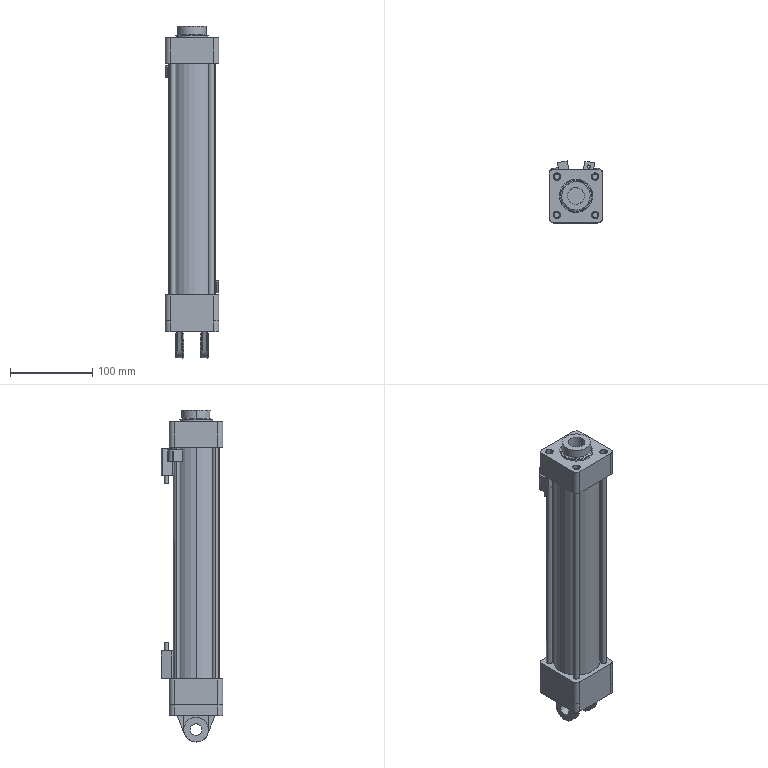Part | STEP file | MDBD50-250-A56 (Barrel) | 1 solid | 270 faces | box 65.01 x 74.997 x 403 mm | volume 1011039 mm3 | plane 145 | cylinder 94 | cone 16 | spline 15 | commonest cylinder face diameters 9 x28 12 x12 6.47 x8 7.2 x8 29.98 x8 4 x4